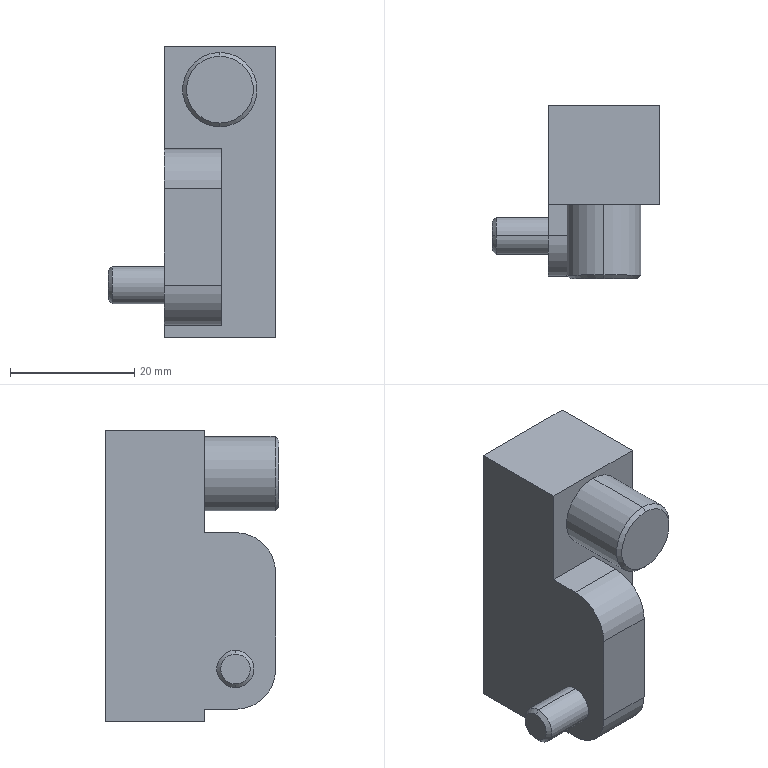Part | NX | features BREP 1 | 1 solid | 22 faces | box 27 x 28 x 47 mm | volume 17986 mm3 | plane 12 | cylinder 6 | cone 4 | commonest cylinder face diameters 6 x2 12 x2 13 x2
STEP:
#1=CARTESIAN_POINT('',(9.,-7.,11.114));
#2=VERTEX_POINT('',#1);
#3=CARTESIAN_POINT('',(9.,-7.,21.887));
#4=VERTEX_POINT('',#3);
#5=CARTESIAN_POINT('',(9.,-7.,16.5));
#6=DIRECTION('',(0.,1.,0.));
#7=DIRECTION('',(0.,0.,-1.));
#8=AXIS2_PLACEMENT_3D('',#5,#6,#7);
#9=CIRCLE('',#8,5.386);
#10=EDGE_CURVE('',#2,#4,#9,.T.);
#11=ORIENTED_EDGE('',*,*,#10,.T.);
#12=CARTESIAN_POINT('',(9.,-6.386,22.5));
#13=VERTEX_POINT('',#12);
#14=CARTESIAN_POINT('',(9.,-6.386,22.5));
#15=DIRECTION('',(0.,-0.7071,-0.7071));
#16=VECTOR('',#15,1000.);
#17=LINE('',#14,#16);
#18=EDGE_CURVE('',#13,#4,#17,.T.);
#19=ORIENTED_EDGE('',*,*,#18,.F.);
#20=CARTESIAN_POINT('',(9.,-6.386,10.5));
#21=VERTEX_POINT('',#20);
#22=CARTESIAN_POINT('',(9.,-6.386,16.5));
#23=DIRECTION('',(0.,1.,0.));
#24=DIRECTION('',(0.,0.,-1.));
#25=AXIS2_PLACEMENT_3D('',#22,#23,#24);
#26=CIRCLE('',#25,6.);
#27=EDGE_CURVE('',#21,#13,#26,.T.);
#28=ORIENTED_EDGE('',*,*,#27,.F.);
#29=CARTESIAN_POINT('',(9.,-6.386,10.5));
#30=DIRECTION('',(0.,-0.7071,0.7071));
#31=VECTOR('',#30,1000.);
#32=LINE('',#29,#31);
#33=EDGE_CURVE('',#21,#2,#32,.T.);
#34=ORIENTED_EDGE('',*,*,#33,.T.);
#35=EDGE_LOOP('',(#11,#19,#28,#34));
#36=FACE_BOUND('',#35,.T.);
#37=CARTESIAN_POINT('',(9.,-7.052,16.5));
#38=DIRECTION('',(0.,1.,0.));
#39=DIRECTION('',(0.,0.,1.));
#40=AXIS2_PLACEMENT_3D('',#37,#38,#39);
#41=CONICAL_SURFACE('',#40,5.335,0.7854);
#42=ADVANCED_FACE('',(#36),#41,.T.);
#43=ORIENTED_EDGE('',*,*,#10,.F.);
#44=CARTESIAN_POINT('',(9.,-7.,16.5));
#45=DIRECTION('',(0.,1.,0.));
#46=DIRECTION('',(0.,0.,1.));
#47=AXIS2_PLACEMENT_3D('',#44,#45,#46);
#48=CIRCLE('',#47,5.386);
#49=EDGE_CURVE('',#4,#2,#48,.T.);
#50=ORIENTED_EDGE('',*,*,#49,.F.);
#51=EDGE_LOOP('',(#43,#50));
#52=FACE_BOUND('',#51,.T.);
#53=CARTESIAN_POINT('',(14.386,-7.,16.5));
#54=DIRECTION('',(0.,1.,0.));
#55=DIRECTION('',(0.,0.,1.));
#56=AXIS2_PLACEMENT_3D('',#53,#54,#55);
#57=PLANE('',#56);
#58=ADVANCED_FACE('',(#52),#57,.F.);
#59=ORIENTED_EDGE('',*,*,#18,.T.);
#60=ORIENTED_EDGE('',*,*,#49,.T.);
#61=ORIENTED_EDGE('',*,*,#33,.F.);
#62=CARTESIAN_POINT('',(9.,-6.386,16.5));
#63=DIRECTION('',(0.,1.,0.));
#64=DIRECTION('',(0.,0.,1.));
#65=AXIS2_PLACEMENT_3D('',#62,#63,#64);
#66=CIRCLE('',#65,6.);
#67=EDGE_CURVE('',#13,#21,#66,.T.);
#68=ORIENTED_EDGE('',*,*,#67,.F.);
#69=EDGE_LOOP('',(#59,#60,#61,#68));
#70=FACE_BOUND('',#69,.T.);
#71=CARTESIAN_POINT('',(9.,-7.052,16.5));
#72=DIRECTION('',(0.,1.,0.));
#73=DIRECTION('',(0.,0.,1.));
#74=AXIS2_PLACEMENT_3D('',#71,#72,#73);
#75=CONICAL_SURFACE('',#74,5.335,0.7854);
#76=ADVANCED_FACE('',(#70),#75,.T.);
#77=CARTESIAN_POINT('',(9.,5.,22.5));
#78=VERTEX_POINT('',#77);
#79=CARTESIAN_POINT('',(9.,5.,22.5));
#80=DIRECTION('',(0.,-1.,0.));
#81=VECTOR('',#80,1000.);
#82=LINE('',#79,#81);
#83=EDGE_CURVE('',#13,#78,#82,.F.);
#84=ORIENTED_EDGE('',*,*,#83,.F.);
#85=ORIENTED_EDGE('',*,*,#67,.T.);
#86=CARTESIAN_POINT('',(9.,5.,10.5));
#87=VERTEX_POINT('',#86);
#88=CARTESIAN_POINT('',(9.,5.,10.5));
#89=DIRECTION('',(0.,-1.,0.));
#90=VECTOR('',#89,1000.);
#91=LINE('',#88,#90);
#92=EDGE_CURVE('',#21,#87,#91,.F.);
#93=ORIENTED_EDGE('',*,*,#92,.T.);
#94=CARTESIAN_POINT('',(9.,5.,16.5));
#95=DIRECTION('',(0.,-1.,0.));
#96=DIRECTION('',(0.,0.,-1.));
#97=AXIS2_PLACEMENT_3D('',#94,#95,#96);
#98=CIRCLE('',#97,6.);
#99=EDGE_CURVE('',#87,#78,#98,.T.);
#100=ORIENTED_EDGE('',*,*,#99,.T.);
#101=EDGE_LOOP('',(#84,#85,#93,#100));
#102=FACE_BOUND('',#101,.T.);
#103=CARTESIAN_POINT('',(9.,-7.,16.5));
#104=DIRECTION('',(0.,1.,0.));
#105=DIRECTION('',(0.,0.,1.));
#106=AXIS2_PLACEMENT_3D('',#103,#104,#105);
#107=CYLINDRICAL_SURFACE('',#106,6.);
#108=ADVANCED_FACE('',(#102),#107,.T.);
#109=ORIENTED_EDGE('',*,*,#27,.T.);
#110=ORIENTED_EDGE('',*,*,#83,.T.);
#111=CARTESIAN_POINT('',(9.,5.,16.5));
#112=DIRECTION('',(0.,-1.,0.));
#113=DIRECTION('',(0.,0.,1.));
#114=AXIS2_PLACEMENT_3D('',#111,#112,#113);
#115=CIRCLE('',#114,6.);
#116=EDGE_CURVE('',#78,#87,#115,.T.);
#117=ORIENTED_EDGE('',*,*,#116,.T.);
#118=ORIENTED_EDGE('',*,*,#92,.F.);
#119=EDGE_LOOP('',(#109,#110,#117,#118));
#120=FACE_BOUND('',#119,.T.);
#121=CARTESIAN_POINT('',(9.,-7.,16.5));
#122=DIRECTION('',(0.,1.,0.));
#123=DIRECTION('',(0.,0.,1.));
#124=AXIS2_PLACEMENT_3D('',#121,#122,#123);
#125=CYLINDRICAL_SURFACE('',#124,6.);
#126=ADVANCED_FACE('',(#120),#125,.T.);
#127=CARTESIAN_POINT('',(18.,21.,23.5));
#128=VERTEX_POINT('',#127);
#129=CARTESIAN_POINT('',(18.,5.,23.5));
#130=VERTEX_POINT('',#129);
#131=CARTESIAN_POINT('',(18.,21.,23.5));
#132=DIRECTION('',(0.,-1.,0.));
#133=VECTOR('',#132,1000.);
#134=LINE('',#131,#133);
#135=EDGE_CURVE('',#128,#130,#134,.T.);
#136=ORIENTED_EDGE('',*,*,#135,.F.);
#137=CARTESIAN_POINT('',(0.,21.,23.5));
#138=VERTEX_POINT('',#137);
#139=CARTESIAN_POINT('',(0.,21.,23.5));
#140=DIRECTION('',(1.,0.,0.));
#141=VECTOR('',#140,1000.);
#142=LINE('',#139,#141);
#143=EDGE_CURVE('',#138,#128,#142,.T.);
#144=ORIENTED_EDGE('',*,*,#143,.F.);
#145=CARTESIAN_POINT('',(0.,5.,23.5));
#146=VERTEX_POINT('',#145);
#147=CARTESIAN_POINT('',(0.,5.,23.5));
#148=DIRECTION('',(0.,1.,0.));
#149=VECTOR('',#148,1000.);
#150=LINE('',#147,#149);
#151=EDGE_CURVE('',#146,#138,#150,.T.);
#152=ORIENTED_EDGE('',*,*,#151,.F.);
#153=CARTESIAN_POINT('',(18.,5.,23.5));
#154=DIRECTION('',(-1.,0.,0.));
#155=VECTOR('',#154,1000.);
#156=LINE('',#153,#155);
#157=EDGE_CURVE('',#130,#146,#156,.T.);
#158=ORIENTED_EDGE('',*,*,#157,.F.);
#159=EDGE_LOOP('',(#136,#144,#152,#158));
#160=FACE_BOUND('',#159,.T.);
#161=CARTESIAN_POINT('',(0.,0.,23.5));
#162=DIRECTION('',(0.,0.,-1.));
#163=DIRECTION('',(-1.,0.,0.));
#164=AXIS2_PLACEMENT_3D('',#161,#162,#163);
#165=PLANE('',#164);
#166=ADVANCED_FACE('',(#160),#165,.F.);
#167=CARTESIAN_POINT('',(0.,5.,-23.5));
#168=VERTEX_POINT('',#167);
#169=CARTESIAN_POINT('',(0.,21.,-23.5));
#170=VERTEX_POINT('',#169);
#171=CARTESIAN_POINT('',(0.,5.,-23.5));
#172=DIRECTION('',(0.,1.,0.));
#173=VECTOR('',#172,1000.);
#174=LINE('',#171,#173);
#175=EDGE_CURVE('',#168,#170,#174,.T.);
#176=ORIENTED_EDGE('',*,*,#175,.T.);
#177=CARTESIAN_POINT('',(18.,21.,-23.5));
#178=VERTEX_POINT('',#177);
#179=CARTESIAN_POINT('',(0.,21.,-23.5));
#180=DIRECTION('',(1.,0.,0.));
#181=VECTOR('',#180,1000.);
#182=LINE('',#179,#181);
#183=EDGE_CURVE('',#170,#178,#182,.T.);
#184=ORIENTED_EDGE('',*,*,#183,.T.);
#185=CARTESIAN_POINT('',(18.,5.,-23.5));
#186=VERTEX_POINT('',#185);
#187=CARTESIAN_POINT('',(18.,21.,-23.5));
#188=DIRECTION('',(0.,-1.,0.));
#189=VECTOR('',#188,1000.);
#190=LINE('',#187,#189);
#191=EDGE_CURVE('',#178,#186,#190,.T.);
#192=ORIENTED_EDGE('',*,*,#191,.T.);
#193=CARTESIAN_POINT('',(18.,5.,-23.5));
#194=DIRECTION('',(-1.,0.,0.));
#195=VECTOR('',#194,1000.);
#196=LINE('',#193,#195);
#197=EDGE_CURVE('',#186,#168,#196,.T.);
#198=ORIENTED_EDGE('',*,*,#197,.T.);
#199=EDGE_LOOP('',(#176,#184,#192,#198));
#200=FACE_BOUND('',#199,.T.);
#201=CARTESIAN_POINT('',(0.,0.,-23.5));
#202=DIRECTION('',(0.,0.,-1.));
#203=DIRECTION('',(-1.,0.,0.));
#204=AXIS2_PLACEMENT_3D('',#201,#202,#203);
#205=PLANE('',#204);
#206=ADVANCED_FACE('',(#200),#205,.T.);
#207=CARTESIAN_POINT('',(9.2,-6.5,0.5));
#208=VERTEX_POINT('',#207);
#209=CARTESIAN_POINT('',(9.2,-6.5,-15.));
#210=VERTEX_POINT('',#209);
#211=CARTESIAN_POINT('',(9.2,-6.5,0.5));
#212=DIRECTION('',(0.,0.,-1.));
#213=VECTOR('',#212,1000.);
#214=LINE('',#211,#213);
#215=EDGE_CURVE('',#208,#210,#214,.T.);
#216=ORIENTED_EDGE('',*,*,#215,.T.);
#217=CARTESIAN_POINT('',(9.2,0.,-21.5));
#218=VERTEX_POINT('',#217);
#219=CARTESIAN_POINT('',(9.2,0.,-15.));
#220=DIRECTION('',(-1.,0.,0.));
#221=DIRECTION('',(0.,0.,-1.));
#222=AXIS2_PLACEMENT_3D('',#219,#220,#221);
#223=CIRCLE('',#222,6.5);
#224=EDGE_CURVE('',#218,#210,#223,.T.);
#225=ORIENTED_EDGE('',*,*,#224,.F.);
#226=CARTESIAN_POINT('',(9.2,5.,-21.5));
#227=VERTEX_POINT('',#226);
#228=CARTESIAN_POINT('',(9.2,0.,-21.5));
#229=DIRECTION('',(0.,1.,0.));
#230=VECTOR('',#229,1000.);
#231=LINE('',#228,#230);
#232=EDGE_CURVE('',#218,#227,#231,.T.);
#233=ORIENTED_EDGE('',*,*,#232,.T.);
#234=CARTESIAN_POINT('',(9.2,5.,7.));
#235=VERTEX_POINT('',#234);
#236=CARTESIAN_POINT('',(9.2,5.,-21.5));
#237=DIRECTION('',(0.,0.,1.));
#238=VECTOR('',#237,1000.);
#239=LINE('',#236,#238);
#240=EDGE_CURVE('',#227,#235,#239,.T.);
#241=ORIENTED_EDGE('',*,*,#240,.T.);
#242=CARTESIAN_POINT('',(9.2,0.,7.));
#243=VERTEX_POINT('',#242);
#244=CARTESIAN_POINT('',(9.2,5.,7.));
#245=DIRECTION('',(0.,-1.,0.));
#246=VECTOR('',#245,1000.);
#247=LINE('',#244,#246);
#248=EDGE_CURVE('',#235,#243,#247,.T.);
#249=ORIENTED_EDGE('',*,*,#248,.T.);
#250=CARTESIAN_POINT('',(9.2,0.,0.5));
#251=DIRECTION('',(-1.,0.,0.));
#252=DIRECTION('',(0.,-1.,0.));
#253=AXIS2_PLACEMENT_3D('',#250,#251,#252);
#254=CIRCLE('',#253,6.5);
#255=EDGE_CURVE('',#208,#243,#254,.T.);
#256=ORIENTED_EDGE('',*,*,#255,.F.);
#257=EDGE_LOOP('',(#216,#225,#233,#241,#249,#256));
#258=FACE_BOUND('',#257,.T.);
#259=CARTESIAN_POINT('',(9.2,0.,-15.));
#260=DIRECTION('',(1.,0.,0.));
#261=DIRECTION('',(0.,0.,-1.));
#262=AXIS2_PLACEMENT_3D('',#259,#260,#261);
#263=PLANE('',#262);
#264=ADVANCED_FACE('',(#258),#263,.T.);
#265=CARTESIAN_POINT('',(0.,0.,-21.5));
#266=VERTEX_POINT('',#265);
#267=CARTESIAN_POINT('',(9.2,0.,-21.5));
#268=DIRECTION('',(-1.,0.,0.));
#269=VECTOR('',#268,1000.);
#270=LINE('',#267,#269);
#271=EDGE_CURVE('',#218,#266,#270,.T.);
#272=ORIENTED_EDGE('',*,*,#271,.T.);
#273=CARTESIAN_POINT('',(0.,5.,-21.5));
#274=VERTEX_POINT('',#273);
#275=CARTESIAN_POINT('',(0.,0.,-21.5));
#276=DIRECTION('',(0.,1.,0.));
#277=VECTOR('',#276,1000.);
#278=LINE('',#275,#277);
#279=EDGE_CURVE('',#266,#274,#278,.T.);
#280=ORIENTED_EDGE('',*,*,#279,.T.);
#281=CARTESIAN_POINT('',(0.,5.,-21.5));
#282=DIRECTION('',(1.,0.,0.));
#283=VECTOR('',#282,1000.);
#284=LINE('',#281,#283);
#285=EDGE_CURVE('',#274,#227,#284,.T.);
#286=ORIENTED_EDGE('',*,*,#285,.T.);
#287=ORIENTED_EDGE('',*,*,#232,.F.);
#288=EDGE_LOOP('',(#272,#280,#286,#287));
#289=FACE_BOUND('',#288,.T.);
#290=CARTESIAN_POINT('',(9.2,5.,-21.5));
#291=DIRECTION('',(0.,0.,1.));
#292=DIRECTION('',(1.,0.,0.));
#293=AXIS2_PLACEMENT_3D('',#290,#291,#292);
#294=PLANE('',#293);
#295=ADVANCED_FACE('',(#289),#294,.F.);
#296=CARTESIAN_POINT('',(0.,-6.5,-15.));
#297=VERTEX_POINT('',#296);
#298=CARTESIAN_POINT('',(0.,-6.5,-15.));
#299=DIRECTION('',(1.,0.,0.));
#300=VECTOR('',#299,1000.);
#301=LINE('',#298,#300);
#302=EDGE_CURVE('',#297,#210,#301,.T.);
#303=ORIENTED_EDGE('',*,*,#302,.F.);
#304=CARTESIAN_POINT('',(0.,0.,-15.));
#305=DIRECTION('',(1.,0.,0.));
#306=DIRECTION('',(0.,-1.,0.));
#307=AXIS2_PLACEMENT_3D('',#304,#305,#306);
#308=CIRCLE('',#307,6.5);
#309=EDGE_CURVE('',#297,#266,#308,.T.);
#310=ORIENTED_EDGE('',*,*,#309,.T.);
#311=ORIENTED_EDGE('',*,*,#271,.F.);
#312=ORIENTED_EDGE('',*,*,#224,.T.);
#313=EDGE_LOOP('',(#303,#310,#311,#312));
#314=FACE_BOUND('',#313,.T.);
#315=CARTESIAN_POINT('',(9.2,0.,-15.));
#316=DIRECTION('',(-1.,0.,0.));
#317=DIRECTION('',(0.,0.,1.));
#318=AXIS2_PLACEMENT_3D('',#315,#316,#317);
#319=CYLINDRICAL_SURFACE('',#318,6.5);
#320=ADVANCED_FACE('',(#314),#319,.T.);
#321=CARTESIAN_POINT('',(0.,-6.5,0.5));
#322=VERTEX_POINT('',#321);
#323=CARTESIAN_POINT('',(9.2,-6.5,0.5));
#324=DIRECTION('',(-1.,0.,0.));
#325=VECTOR('',#324,1000.);
#326=LINE('',#323,#325);
#327=EDGE_CURVE('',#208,#322,#326,.T.);
#328=ORIENTED_EDGE('',*,*,#327,.T.);
#329=CARTESIAN_POINT('',(0.,-6.5,0.5));
#330=DIRECTION('',(0.,0.,-1.));
#331=VECTOR('',#330,1000.);
#332=LINE('',#329,#331);
#333=EDGE_CURVE('',#322,#297,#332,.T.);
#334=ORIENTED_EDGE('',*,*,#333,.T.);
#335=ORIENTED_EDGE('',*,*,#302,.T.);
#336=ORIENTED_EDGE('',*,*,#215,.F.);
#337=EDGE_LOOP('',(#328,#334,#335,#336));
#338=FACE_BOUND('',#337,.T.);
#339=CARTESIAN_POINT('',(9.2,-6.5,-15.));
#340=DIRECTION('',(0.,1.,0.));
#341=DIRECTION('',(0.,0.,1.));
#342=AXIS2_PLACEMENT_3D('',#339,#340,#341);
#343=PLANE('',#342);
#344=ADVANCED_FACE('',(#338),#343,.F.);
#345=CARTESIAN_POINT('',(0.,0.,7.));
#346=VERTEX_POINT('',#345);
#347=CARTESIAN_POINT('',(0.,0.,7.));
#348=DIRECTION('',(1.,0.,0.));
#349=VECTOR('',#348,1000.);
#350=LINE('',#347,#349);
#351=EDGE_CURVE('',#346,#243,#350,.T.);
#352=ORIENTED_EDGE('',*,*,#351,.F.);
#353=CARTESIAN_POINT('',(0.,0.,0.5));
#354=DIRECTION('',(1.,0.,0.));
#355=DIRECTION('',(0.,0.,1.));
#356=AXIS2_PLACEMENT_3D('',#353,#354,#355);
#357=CIRCLE('',#356,6.5);
#358=EDGE_CURVE('',#346,#322,#357,.T.);
#359=ORIENTED_EDGE('',*,*,#358,.T.);
#360=ORIENTED_EDGE('',*,*,#327,.F.);
#361=ORIENTED_EDGE('',*,*,#255,.T.);
#362=EDGE_LOOP('',(#352,#359,#360,#361));
#363=FACE_BOUND('',#362,.T.);
#364=CARTESIAN_POINT('',(9.2,0.,0.5));
#365=DIRECTION('',(-1.,0.,0.));
#366=DIRECTION('',(0.,0.,1.));
#367=AXIS2_PLACEMENT_3D('',#364,#365,#366);
#368=CYLINDRICAL_SURFACE('',#367,6.5);
#369=ADVANCED_FACE('',(#363),#368,.T.);
#370=CARTESIAN_POINT('',(0.,5.,7.));
#371=VERTEX_POINT('',#370);
#372=CARTESIAN_POINT('',(0.,5.,7.));
#373=DIRECTION('',(1.,0.,0.));
#374=VECTOR('',#373,1000.);
#375=LINE('',#372,#374);
#376=EDGE_CURVE('',#371,#235,#375,.T.);
#377=ORIENTED_EDGE('',*,*,#376,.F.);
#378=CARTESIAN_POINT('',(0.,5.,7.));
#379=DIRECTION('',(0.,-1.,0.));
#380=VECTOR('',#379,1000.);
#381=LINE('',#378,#380);
#382=EDGE_CURVE('',#371,#346,#381,.T.);
#383=ORIENTED_EDGE('',*,*,#382,.T.);
#384=ORIENTED_EDGE('',*,*,#351,.T.);
#385=ORIENTED_EDGE('',*,*,#248,.F.);
#386=EDGE_LOOP('',(#377,#383,#384,#385));
#387=FACE_BOUND('',#386,.T.);
#388=CARTESIAN_POINT('',(9.2,0.,7.));
#389=DIRECTION('',(0.,0.,-1.));
#390=DIRECTION('',(-1.,0.,0.));
#391=AXIS2_PLACEMENT_3D('',#388,#389,#390);
#392=PLANE('',#391);
#393=ADVANCED_FACE('',(#387),#392,.F.);
#394=ORIENTED_EDGE('',*,*,#99,.F.);
#395=ORIENTED_EDGE('',*,*,#116,.F.);
#396=EDGE_LOOP('',(#394,#395));
#397=FACE_BOUND('',#396,.T.);
#398=CARTESIAN_POINT('',(0.,5.,23.5));
#399=DIRECTION('',(0.,0.,-1.));
#400=VECTOR('',#399,1000.);
#401=LINE('',#398,#400);
#402=EDGE_CURVE('',#146,#371,#401,.T.);
#403=ORIENTED_EDGE('',*,*,#402,.T.);
#404=ORIENTED_EDGE('',*,*,#376,.T.);
#405=ORIENTED_EDGE('',*,*,#240,.F.);
#406=ORIENTED_EDGE('',*,*,#285,.F.);
#407=CARTESIAN_POINT('',(0.,5.,-21.5));
#408=DIRECTION('',(0.,0.,-1.));
#409=VECTOR('',#408,1000.);
#410=LINE('',#407,#409);
#411=EDGE_CURVE('',#274,#168,#410,.T.);
#412=ORIENTED_EDGE('',*,*,#411,.T.);
#413=ORIENTED_EDGE('',*,*,#197,.F.);
#414=CARTESIAN_POINT('',(18.,5.,23.5));
#415=DIRECTION('',(0.,0.,-1.));
#416=VECTOR('',#415,1000.);
#417=LINE('',#414,#416);
#418=EDGE_CURVE('',#130,#186,#417,.T.);
#419=ORIENTED_EDGE('',*,*,#418,.F.);
#420=ORIENTED_EDGE('',*,*,#157,.T.);
#421=EDGE_LOOP('',(#403,#404,#405,#406,#412,#413,#419,#420));
#422=FACE_BOUND('',#421,.T.);
#423=CARTESIAN_POINT('',(0.,5.,-23.5));
#424=DIRECTION('',(0.,1.,0.));
#425=DIRECTION('',(0.,0.,1.));
#426=AXIS2_PLACEMENT_3D('',#423,#424,#425);
#427=PLANE('',#426);
#428=ADVANCED_FACE('',(#397,#422),#427,.F.);
#429=ORIENTED_EDGE('',*,*,#135,.T.);
#430=ORIENTED_EDGE('',*,*,#418,.T.);
#431=ORIENTED_EDGE('',*,*,#191,.F.);
#432=CARTESIAN_POINT('',(18.,21.,23.5));
#433=DIRECTION('',(0.,0.,-1.));
#434=VECTOR('',#433,1000.);
#435=LINE('',#432,#434);
#436=EDGE_CURVE('',#128,#178,#435,.T.);
#437=ORIENTED_EDGE('',*,*,#436,.F.);
#438=EDGE_LOOP('',(#429,#430,#431,#437));
#439=FACE_BOUND('',#438,.T.);
#440=CARTESIAN_POINT('',(18.,5.,-23.5));
#441=DIRECTION('',(-1.,0.,0.));
#442=DIRECTION('',(0.,0.,1.));
#443=AXIS2_PLACEMENT_3D('',#440,#441,#442);
#444=PLANE('',#443);
#445=ADVANCED_FACE('',(#439),#444,.F.);
#446=ORIENTED_EDGE('',*,*,#143,.T.);
#447=ORIENTED_EDGE('',*,*,#436,.T.);
#448=ORIENTED_EDGE('',*,*,#183,.F.);
#449=CARTESIAN_POINT('',(0.,21.,23.5));
#450=DIRECTION('',(0.,0.,-1.));
#451=VECTOR('',#450,1000.);
#452=LINE('',#449,#451);
#453=EDGE_CURVE('',#138,#170,#452,.T.);
#454=ORIENTED_EDGE('',*,*,#453,.F.);
#455=EDGE_LOOP('',(#446,#447,#448,#454));
#456=FACE_BOUND('',#455,.T.);
#457=CARTESIAN_POINT('',(18.,21.,-23.5));
#458=DIRECTION('',(0.,-1.,0.));
#459=DIRECTION('',(0.,0.,-1.));
#460=AXIS2_PLACEMENT_3D('',#457,#458,#459);
#461=PLANE('',#460);
#462=ADVANCED_FACE('',(#456),#461,.F.);
#463=CARTESIAN_POINT('',(0.,0.,-12.));
#464=VERTEX_POINT('',#463);
#465=CARTESIAN_POINT('',(0.,0.,-18.));
#466=VERTEX_POINT('',#465);
#467=CARTESIAN_POINT('',(0.,0.,-15.));
#468=DIRECTION('',(-1.,0.,0.));
#469=DIRECTION('',(0.,0.,1.));
#470=AXIS2_PLACEMENT_3D('',#467,#468,#469);
#471=CIRCLE('',#470,3.);
#472=EDGE_CURVE('',#464,#466,#471,.T.);
#473=ORIENTED_EDGE('',*,*,#472,.F.);
#474=CARTESIAN_POINT('',(0.,0.,-15.));
#475=DIRECTION('',(-1.,0.,0.));
#476=DIRECTION('',(0.,0.,-1.));
#477=AXIS2_PLACEMENT_3D('',#474,#475,#476);
#478=CIRCLE('',#477,3.);
#479=EDGE_CURVE('',#466,#464,#478,.T.);
#480=ORIENTED_EDGE('',*,*,#479,.F.);
#481=EDGE_LOOP('',(#473,#480));
#482=FACE_BOUND('',#481,.T.);
#483=ORIENTED_EDGE('',*,*,#151,.T.);
#484=ORIENTED_EDGE('',*,*,#453,.T.);
#485=ORIENTED_EDGE('',*,*,#175,.F.);
#486=ORIENTED_EDGE('',*,*,#411,.F.);
#487=ORIENTED_EDGE('',*,*,#279,.F.);
#488=ORIENTED_EDGE('',*,*,#309,.F.);
#489=ORIENTED_EDGE('',*,*,#333,.F.);
#490=ORIENTED_EDGE('',*,*,#358,.F.);
#491=ORIENTED_EDGE('',*,*,#382,.F.);
#492=ORIENTED_EDGE('',*,*,#402,.F.);
#493=EDGE_LOOP('',(#483,#484,#485,#486,#487,#488,#489,#490,#491,#492));
#494=FACE_BOUND('',#493,.T.);
#495=CARTESIAN_POINT('',(0.,21.,-23.5));
#496=DIRECTION('',(1.,0.,0.));
#497=DIRECTION('',(0.,0.,-1.));
#498=AXIS2_PLACEMENT_3D('',#495,#496,#497);
#499=PLANE('',#498);
#500=ADVANCED_FACE('',(#482,#494),#499,.F.);
#501=CARTESIAN_POINT('',(-9.,0.,-12.614));
#502=VERTEX_POINT('',#501);
#503=CARTESIAN_POINT('',(-9.,0.,-17.387));
#504=VERTEX_POINT('',#503);
#505=CARTESIAN_POINT('',(-9.,0.,-15.));
#506=DIRECTION('',(1.,0.,0.));
#507=DIRECTION('',(0.,0.,1.));
#508=AXIS2_PLACEMENT_3D('',#505,#506,#507);
#509=CIRCLE('',#508,2.386);
#510=EDGE_CURVE('',#502,#504,#509,.T.);
#511=ORIENTED_EDGE('',*,*,#510,.T.);
#512=CARTESIAN_POINT('',(-8.386,0.,-18.));
#513=VERTEX_POINT('',#512);
#514=CARTESIAN_POINT('',(-8.386,0.,-18.));
#515=DIRECTION('',(-0.7071,0.,0.7071));
#516=VECTOR('',#515,1000.);
#517=LINE('',#514,#516);
#518=EDGE_CURVE('',#504,#513,#517,.F.);
#519=ORIENTED_EDGE('',*,*,#518,.T.);
#520=CARTESIAN_POINT('',(-8.386,0.,-12.));
#521=VERTEX_POINT('',#520);
#522=CARTESIAN_POINT('',(-8.386,0.,-15.));
#523=DIRECTION('',(1.,0.,0.));
#524=DIRECTION('',(0.,0.,1.));
#525=AXIS2_PLACEMENT_3D('',#522,#523,#524);
#526=CIRCLE('',#525,3.);
#527=EDGE_CURVE('',#521,#513,#526,.T.);
#528=ORIENTED_EDGE('',*,*,#527,.F.);
#529=CARTESIAN_POINT('',(-8.386,0.,-12.));
#530=DIRECTION('',(-0.7071,0.,-0.7071));
#531=VECTOR('',#530,1000.);
#532=LINE('',#529,#531);
#533=EDGE_CURVE('',#502,#521,#532,.F.);
#534=ORIENTED_EDGE('',*,*,#533,.F.);
#535=EDGE_LOOP('',(#511,#519,#528,#534));
#536=FACE_BOUND('',#535,.T.);
#537=CARTESIAN_POINT('',(-9.052,0.,-15.));
#538=DIRECTION('',(1.,0.,0.));
#539=DIRECTION('',(0.,0.,-1.));
#540=AXIS2_PLACEMENT_3D('',#537,#538,#539);
#541=CONICAL_SURFACE('',#540,2.335,0.7854);
#542=ADVANCED_FACE('',(#536),#541,.T.);
#543=ORIENTED_EDGE('',*,*,#510,.F.);
#544=CARTESIAN_POINT('',(-9.,0.,-15.));
#545=DIRECTION('',(1.,0.,0.));
#546=DIRECTION('',(0.,0.,-1.));
#547=AXIS2_PLACEMENT_3D('',#544,#545,#546);
#548=CIRCLE('',#547,2.386);
#549=EDGE_CURVE('',#504,#502,#548,.T.);
#550=ORIENTED_EDGE('',*,*,#549,.F.);
#551=EDGE_LOOP('',(#543,#550));
#552=FACE_BOUND('',#551,.T.);
#553=CARTESIAN_POINT('',(-9.,-2.386,-15.));
#554=DIRECTION('',(1.,0.,0.));
#555=DIRECTION('',(0.,0.,-1.));
#556=AXIS2_PLACEMENT_3D('',#553,#554,#555);
#557=PLANE('',#556);
#558=ADVANCED_FACE('',(#552),#557,.F.);
#559=ORIENTED_EDGE('',*,*,#518,.F.);
#560=ORIENTED_EDGE('',*,*,#549,.T.);
#561=ORIENTED_EDGE('',*,*,#533,.T.);
#562=CARTESIAN_POINT('',(-8.386,0.,-15.));
#563=DIRECTION('',(1.,0.,0.));
#564=DIRECTION('',(0.,0.,-1.));
#565=AXIS2_PLACEMENT_3D('',#562,#563,#564);
#566=CIRCLE('',#565,3.);
#567=EDGE_CURVE('',#513,#521,#566,.T.);
#568=ORIENTED_EDGE('',*,*,#567,.F.);
#569=EDGE_LOOP('',(#559,#560,#561,#568));
#570=FACE_BOUND('',#569,.T.);
#571=CARTESIAN_POINT('',(-9.052,0.,-15.));
#572=DIRECTION('',(1.,0.,0.));
#573=DIRECTION('',(0.,0.,-1.));
#574=AXIS2_PLACEMENT_3D('',#571,#572,#573);
#575=CONICAL_SURFACE('',#574,2.335,0.7854);
#576=ADVANCED_FACE('',(#570),#575,.T.);
#577=CARTESIAN_POINT('',(0.,0.,-18.));
#578=DIRECTION('',(-1.,0.,0.));
#579=VECTOR('',#578,1000.);
#580=LINE('',#577,#579);
#581=EDGE_CURVE('',#466,#513,#580,.T.);
#582=ORIENTED_EDGE('',*,*,#581,.T.);
#583=ORIENTED_EDGE('',*,*,#567,.T.);
#584=CARTESIAN_POINT('',(0.,0.,-12.));
#585=DIRECTION('',(-1.,0.,0.));
#586=VECTOR('',#585,1000.);
#587=LINE('',#584,#586);
#588=EDGE_CURVE('',#464,#521,#587,.T.);
#589=ORIENTED_EDGE('',*,*,#588,.F.);
#590=ORIENTED_EDGE('',*,*,#472,.T.);
#591=EDGE_LOOP('',(#582,#583,#589,#590));
#592=FACE_BOUND('',#591,.T.);
#593=CARTESIAN_POINT('',(-9.,0.,-15.));
#594=DIRECTION('',(1.,0.,0.));
#595=DIRECTION('',(0.,0.,-1.));
#596=AXIS2_PLACEMENT_3D('',#593,#594,#595);
#597=CYLINDRICAL_SURFACE('',#596,3.);
#598=ADVANCED_FACE('',(#592),#597,.T.);
#599=ORIENTED_EDGE('',*,*,#527,.T.);
#600=ORIENTED_EDGE('',*,*,#581,.F.);
#601=ORIENTED_EDGE('',*,*,#479,.T.);
#602=ORIENTED_EDGE('',*,*,#588,.T.);
#603=EDGE_LOOP('',(#599,#600,#601,#602));
#604=FACE_BOUND('',#603,.T.);
#605=CARTESIAN_POINT('',(-9.,0.,-15.));
#606=DIRECTION('',(1.,0.,0.));
#607=DIRECTION('',(0.,0.,-1.));
#608=AXIS2_PLACEMENT_3D('',#605,#606,#607);
#609=CYLINDRICAL_SURFACE('',#608,3.);
#610=ADVANCED_FACE('',(#604),#609,.T.);
#611=CLOSED_SHELL('',(#42,#58,#76,#108,#126,#166,#206,#264,#295,#320,#344,#369,#393,#428,#445,#462,#500,#542,#558,#576,#598,#610));
#612=MANIFOLD_SOLID_BREP('',#611);
#613=(LENGTH_UNIT()NAMED_UNIT(*)SI_UNIT(.MILLI.,.METRE.));
#614=UNCERTAINTY_MEASURE_WITH_UNIT(LENGTH_MEASURE(0.00001),#613,'','');
#615=(NAMED_UNIT(*)PLANE_ANGLE_UNIT()SI_UNIT($,.RADIAN.));
#616=(NAMED_UNIT(*)SI_UNIT($,.STERADIAN.)SOLID_ANGLE_UNIT());
#617=(GEOMETRIC_REPRESENTATION_CONTEXT(3)GLOBAL_UNCERTAINTY_ASSIGNED_CONTEXT((#614))GLOBAL_UNIT_ASSIGNED_CONTEXT((#613,#615,#616))REPRESENTATION_CONTEXT('',''));
#618=ADVANCED_BREP_SHAPE_REPRESENTATION('',(#612),#617);